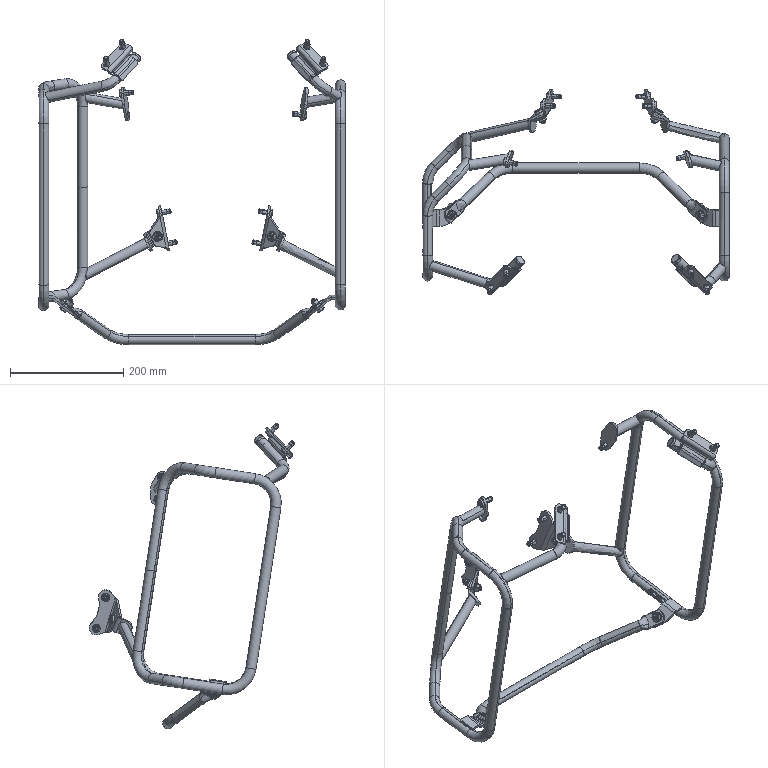Part | SolidWorks | 12 solids | 2059 faces | box 541.7 x 362.675 x 538.827 mm | volume 434535 mm3 | cylinder 664 | spline 603 | plane 339 | cone 252 | torus 189 | sphere 12 | commonest cylinder face diameters 1.586 x112 2.77 x98 8 x86 14 x46 18 x46 6.466 x28